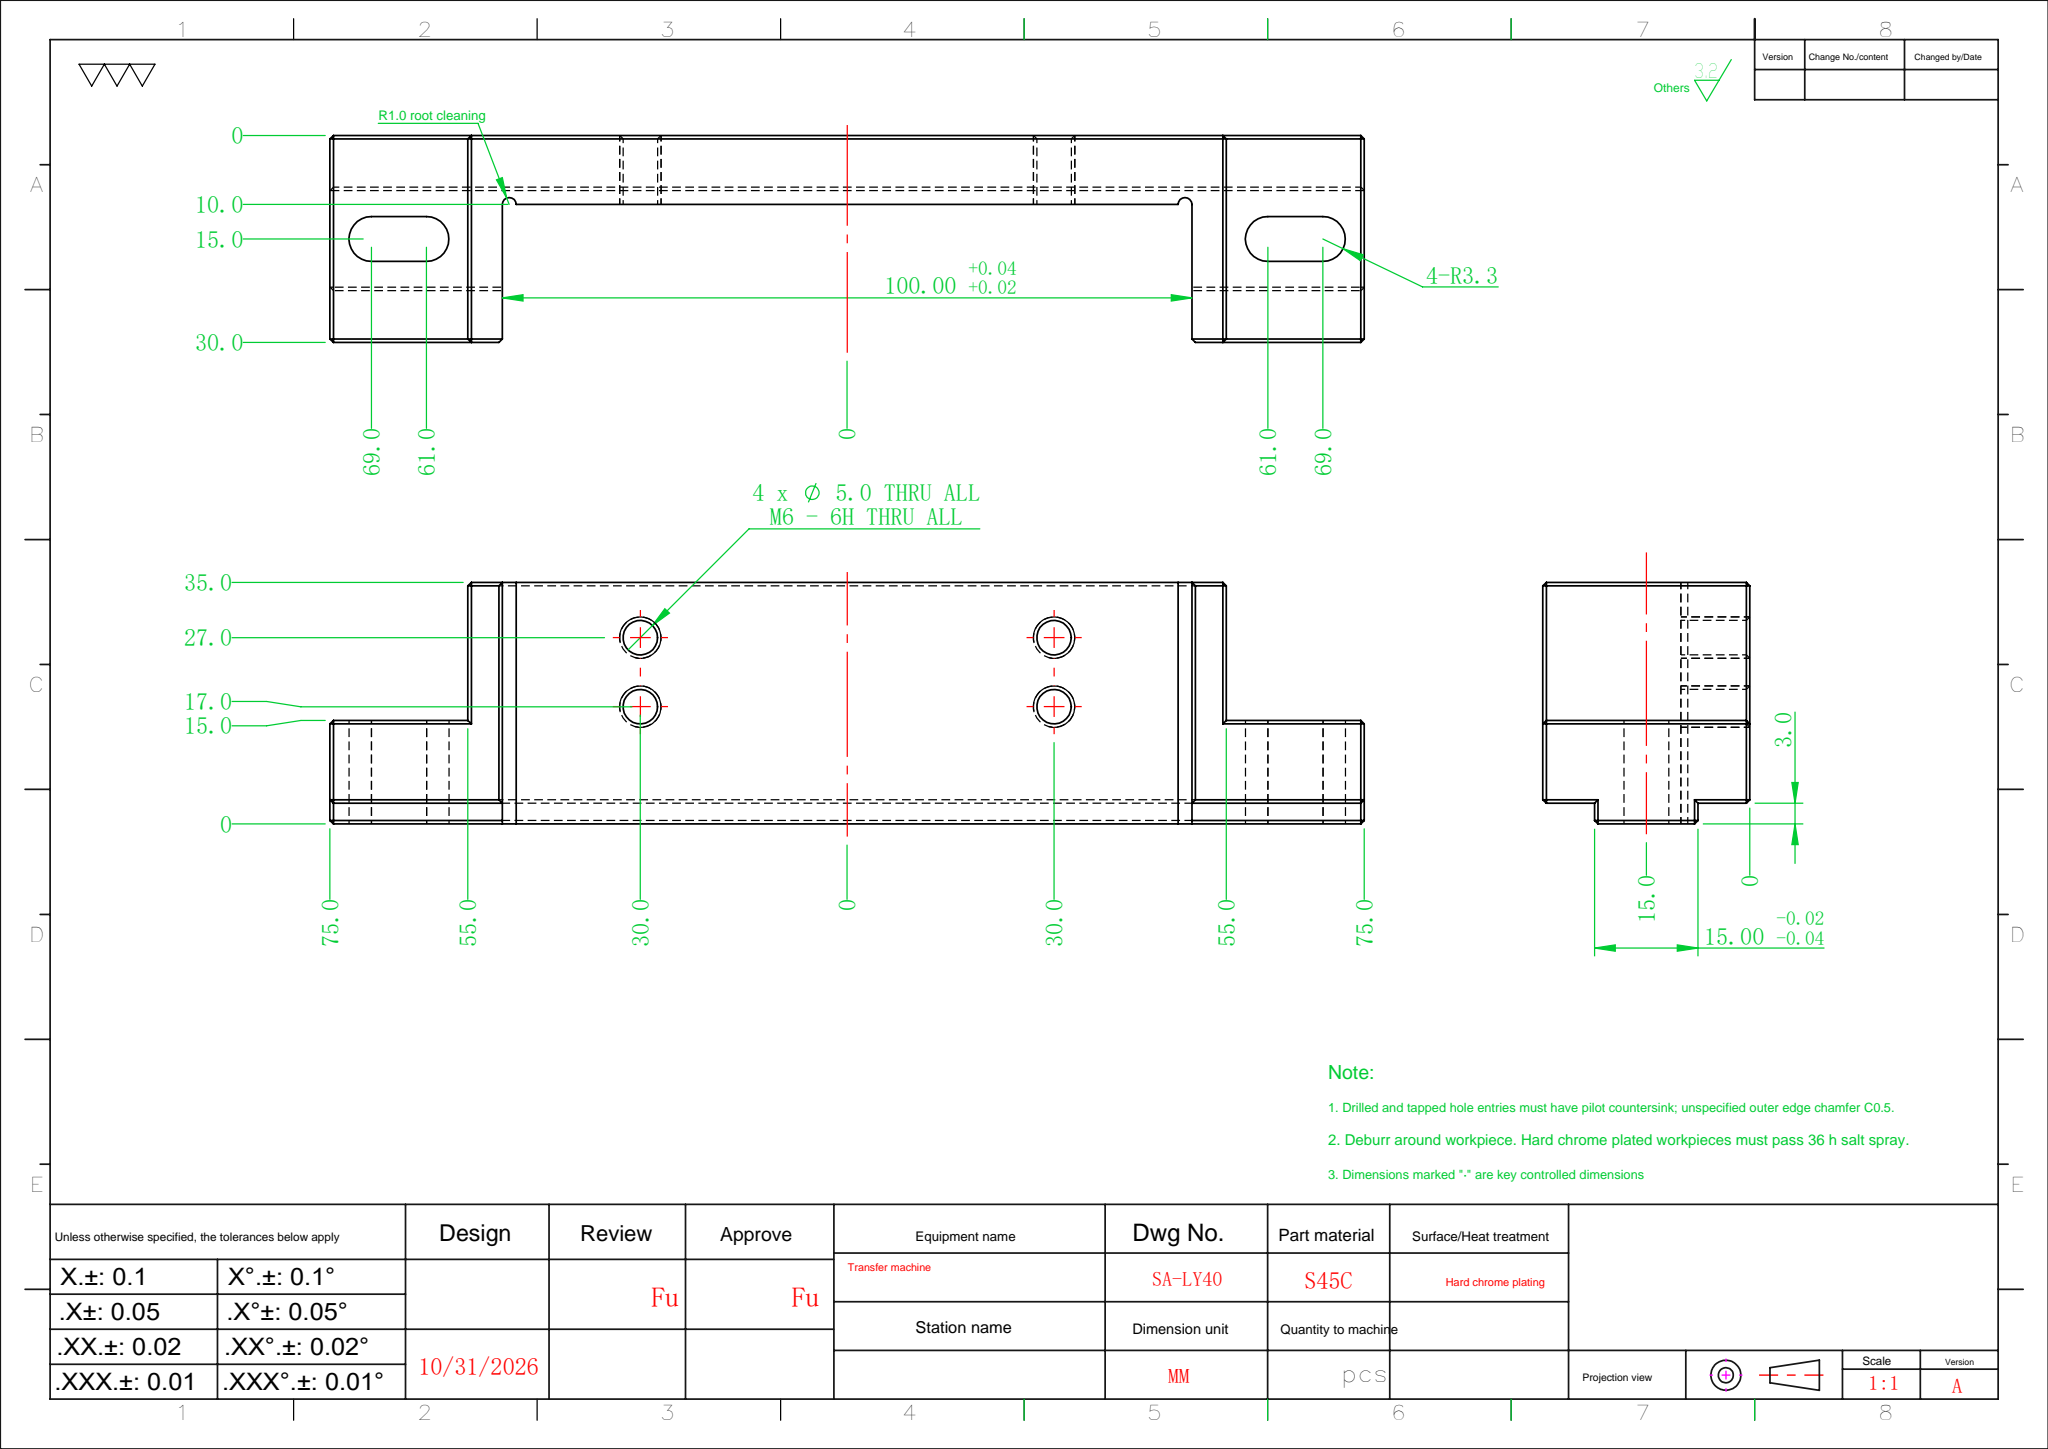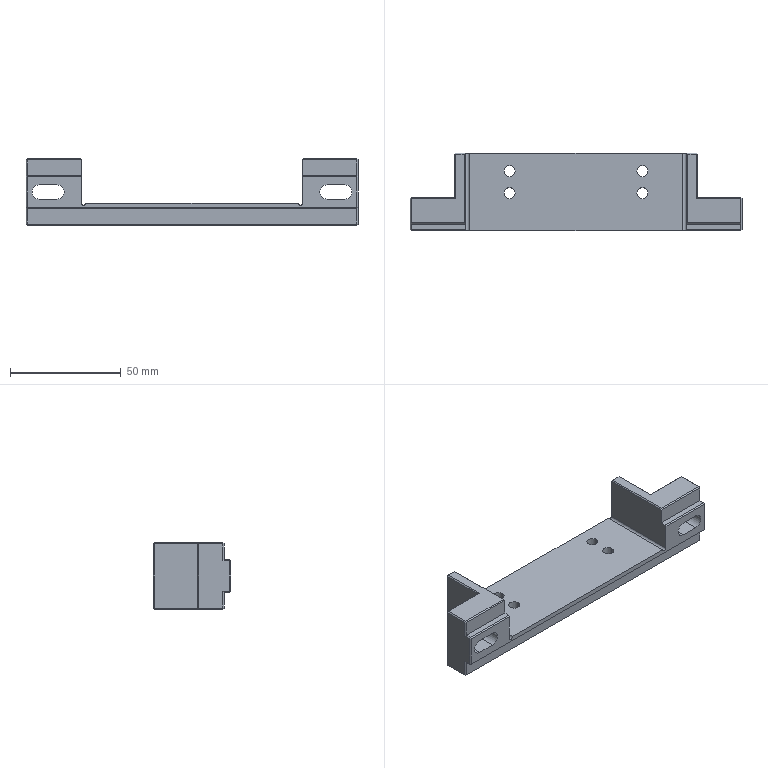Part | SolidWorks | features ICE 4, Chamfer 1, Extrusion 1, HoleWzd 1, LPattern 1 | 1 solid | 99 faces | box 150 x 35 x 30 mm | volume 55419 mm3 | plane 77 | cylinder 14 | cone 8 | commonest cylinder face diameters 5 x8 6.5 x4 2 x2